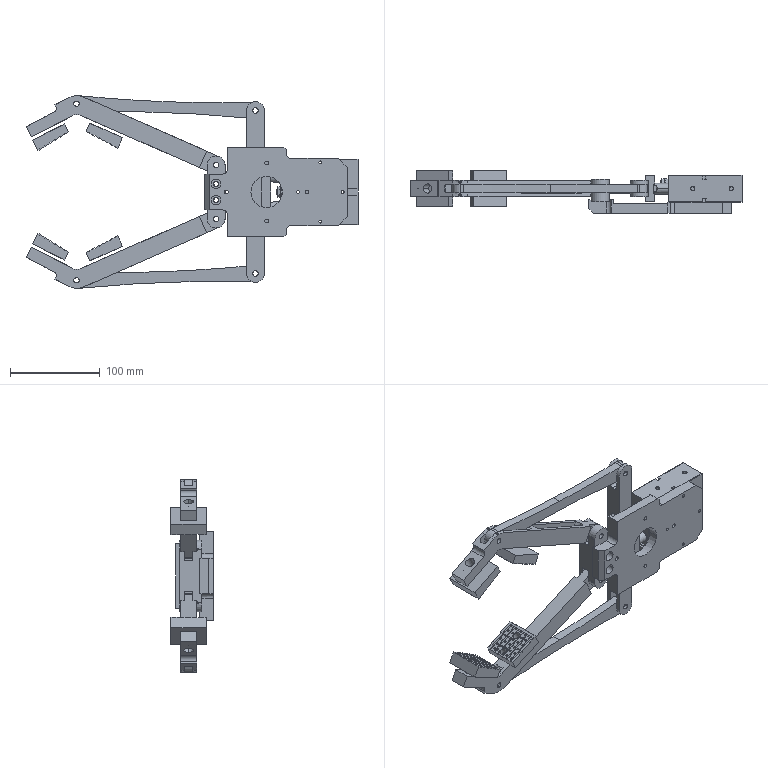Part | SolidWorks | features Simplified 1 | 15 solids | 1705 faces | box 370.752 x 47.5 x 215.235 mm | volume 560908 mm3 | plane 1163 | cylinder 418 | cone 116 | torus 8 | commonest cylinder face diameters 10 x42 6 x38 8 x38 0.4 x30 4.5 x28 2.5 x24